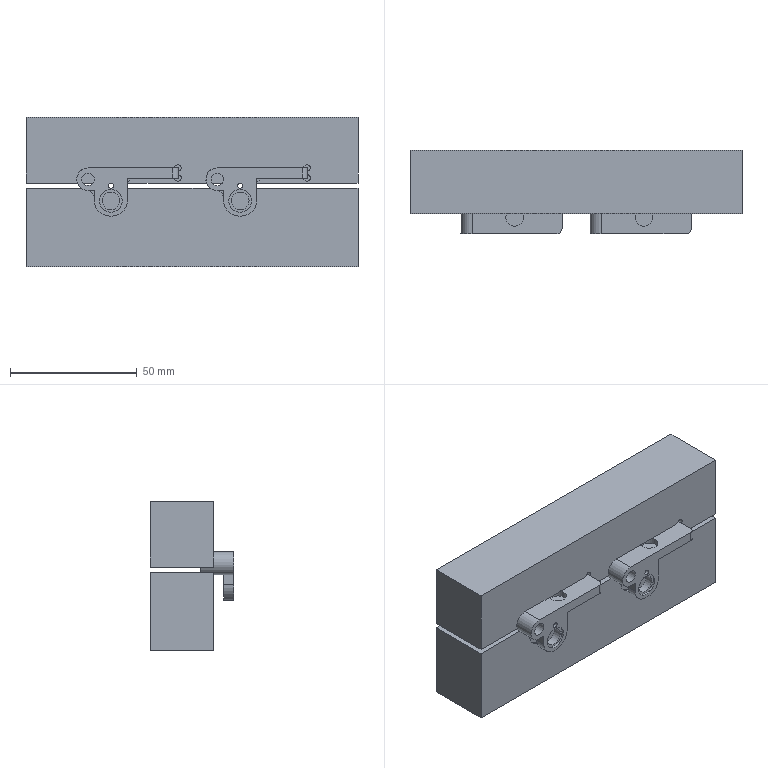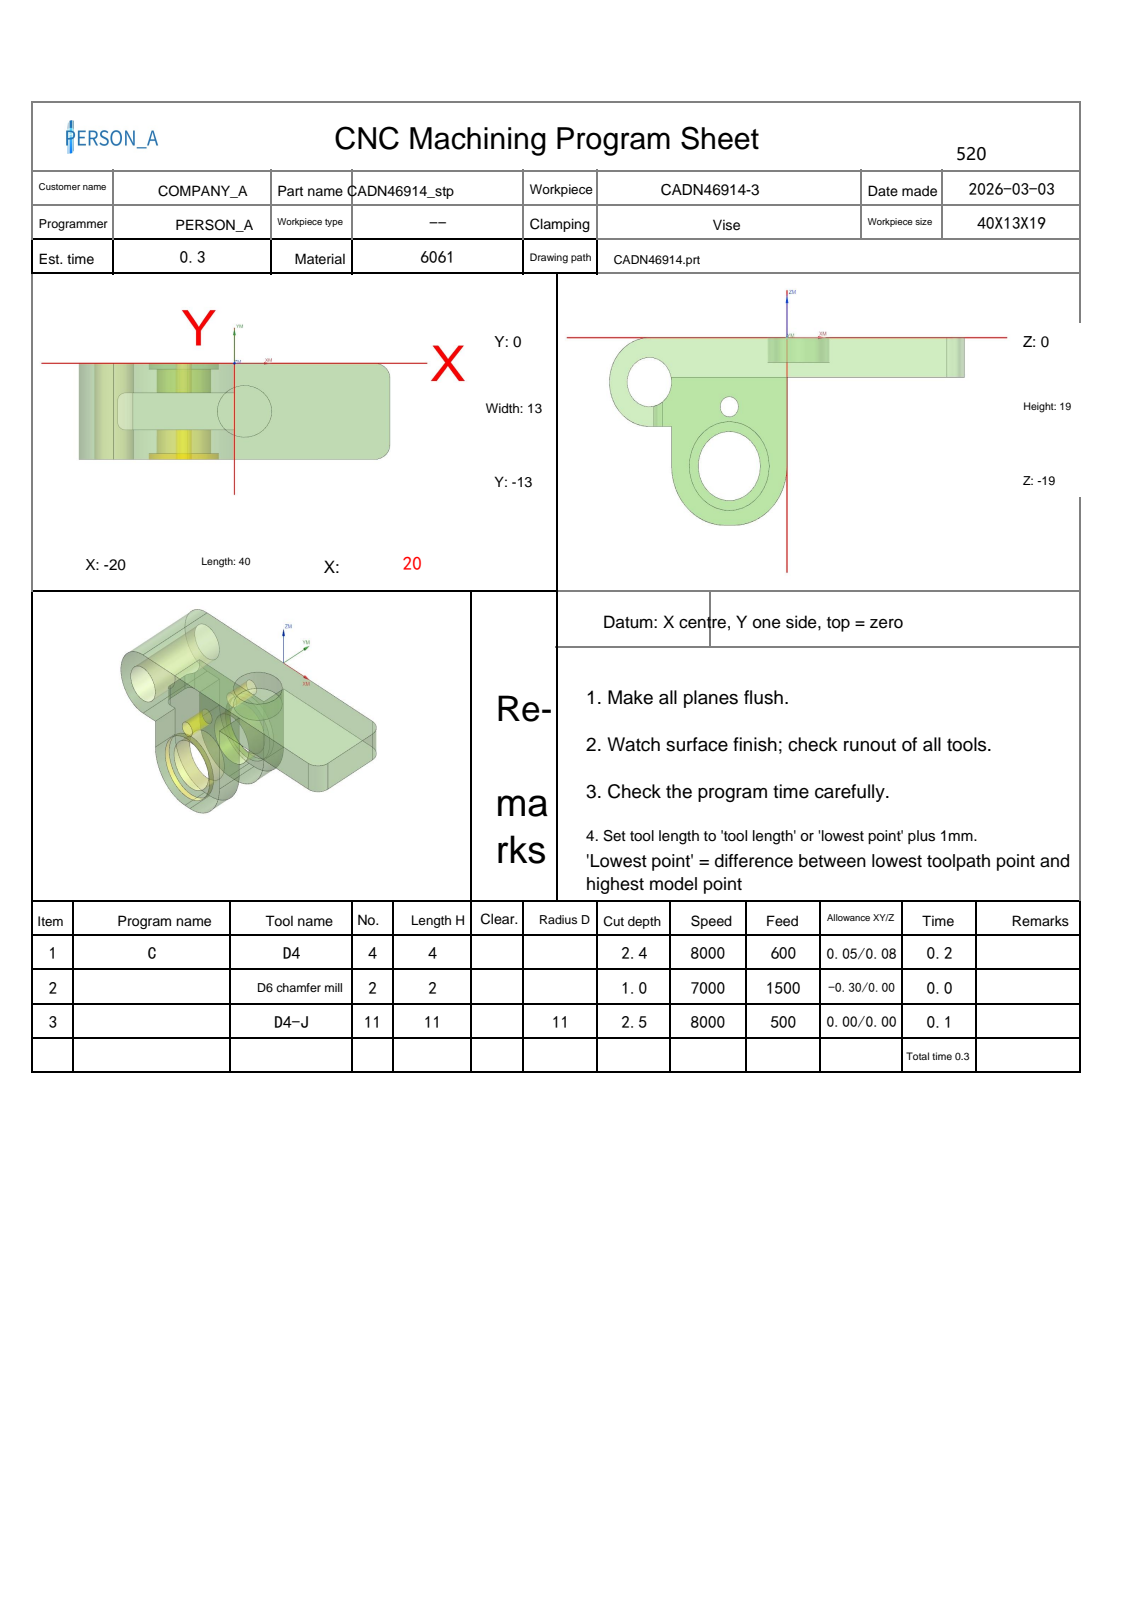NC program | NX | posted by the shop | part box 131 x 33 x 59 mm
Whole program:
%
O0001
(Machine time: 0.90 MIN)
(===Total Tool:3===)
(T4=D4      D=4.   R=0.   D-  H04 Z=-2.44 )
(T2=D6 chamfer mill   D=6.   R=0.   D-  H02 Z=-1.   )
(T11=D4-J   D=4.   R=0.   D11 H11 Z=-2.5  )
G80 G90 G17 G49 G40
G91 G28 Z0
M01
N1 T04 M06
(D4  D=4. R=0. H=04 ce=0.05 di=0.08)
G00 G90 G54 X2.509 Y-5.655 M03 S8000
G43 H04 Z50.
M08
Z.8
G01 X2.124 Y-5.271 Z.771 F600.
X1.596 Y-5.05 Z.742
X1.004 Z.71
X.476 Y-5.271 Z.68
X.071 Y-5.676 Z.65
X-.15 Y-6.204 Z.62
Y-6.796 Z.589
X.207 Y-7.498 Z.548
X.687 Y-7.847 Z.517
X1.004 Y-7.95 Z.5
X1.596 Z.468
X2.124 Y-7.729 Z.439
X2.529 Y-7.324 Z.409
X2.75 Y-6.796 Z.379
Y-6.204 Z.347
X2.529 Y-5.676 Z.317
X2.124 Y-5.271 Z.287
X1.596 Y-5.05 Z.257
X1.004 Z.226
X.476 Y-5.271 Z.196
X.071 Y-5.676 Z.166
X-.15 Y-6.204 Z.136
Y-6.796 Z.105
X.207 Y-7.498 Z.064
X.687 Y-7.847 Z.033
X1.004 Y-7.95 Z.016
X1.3 Z0.0
G03 X2.75 Y-6.5 Z-.068 I0.0 J1.45
X1.3 Y-5.05 Z-.136 I-1.45 J0.0
X-.15 Y-6.5 Z-.203 I0.0 J-1.45
X.447 Y-7.673 Z-.244 I1.45 J0.0
X1.3 Y-7.95 Z-.271 I.853 J1.173
X2.75 Y-6.5 Z-.339 I0.0 J1.45
X1.3 Y-5.05 Z-.407 I-1.45 J0.0
X-.15 Y-6.5 Z-.474 I0.0 J-1.45
X.447 Y-7.673 Z-.515 I1.45 J0.0
X1.3 Y-7.95 Z-.542 I.853 J1.173
X2.75 Y-6.5 Z-.61 I0.0 J1.45
X1.3 Y-5.05 Z-.678 I-1.45 J0.0
X-.15 Y-6.5 Z-.746 I0.0 J-1.45
X.447 Y-7.673 Z-.786 I1.45 J0.0
X1.3 Y-7.95 Z-.813 I.853 J1.173
X2.75 Y-6.5 Z-.881 I0.0 J1.45
X1.3 Y-5.05 Z-.949 I-1.45 J0.0
X-.15 Y-6.5 Z-1.017 I0.0 J-1.45
X.447 Y-7.673 Z-1.057 I1.45 J0.0
X1.3 Y-7.95 Z-1.084 I.853 J1.173
X2.75 Y-6.5 Z-1.152 I0.0 J1.45
X1.3 Y-5.05 Z-1.22 I-1.45 J0.0
X-.15 Y-6.5 Z-1.288 I0.0 J-1.45
X.447 Y-7.673 Z-1.328 I1.45 J0.0
X1.3 Y-7.95 Z-1.356 I.853 J1.173
X2.75 Y-6.5 Z-1.423 I0.0 J1.45
X1.3 Y-5.05 Z-1.491 I-1.45 J0.0
X-.15 Y-6.5 Z-1.559 I0.0 J-1.45
X.447 Y-7.673 Z-1.6 I1.45 J0.0
X1.3 Y-7.95 Z-1.627 I.853 J1.173
X2.75 Y-6.5 Z-1.694 I0.0 J1.45
X1.3 Y-5.05 Z-1.762 I-1.45 J0.0
X-.15 Y-6.5 Z-1.83 I0.0 J-1.45
X.447 Y-7.673 Z-1.871 I1.45 J0.0
X1.3 Y-7.95 Z-1.898 I.853 J1.173
X2.75 Y-6.5 Z-1.966 I0.0 J1.45
X1.3 Y-5.05 Z-2.033 I-1.45 J0.0
X-.15 Y-6.5 Z-2.101 I0.0 J-1.45
X.447 Y-7.673 Z-2.142 I1.45 J0.0
X1.3 Y-7.95 Z-2.169 I.853 J1.173
X2.75 Y-6.5 Z-2.237 I0.0 J1.45
X1.3 Y-5.05 Z-2.304 I-1.45 J0.0
X-.15 Y-6.5 Z-2.372 I0.0 J-1.45
X.447 Y-7.673 Z-2.413 I1.45 J0.0
X1.3 Y-7.95 Z-2.44 I.853 J1.173
X2.75 Y-6.5 I0.0 J1.45
X1.3 Y-5.05 I-1.45 J0.0
X-.15 Y-6.5 I0.0 J-1.45
X1.3 Y-7.95 I1.45 J0.0
X1.695 Y-7.895 I0.0 J1.45
G01 Z-1.64
G00 Z50.
G91 G28 Z0.0
M05
M09
G91 G28 Z0.0
M01
N2 T02 M06
(D6 chamfer mill  D=6. R=0. H=02 ce=-0.30 di=0.00)
G00 G90 G54 X-1.38 Y-5.697 M03 S7000
G43 H02 Z50.
M08
Z2.5
G01 X-1.416 Y-5.806 Z2.458 F1500.
X-1.481 Y-6.15 Z2.331
X-1.503 Y-6.5 Z2.203
X-1.481 Y-6.85 Z2.075
X-1.416 Y-7.194 Z1.948
X-1.308 Y-7.528 Z1.82
X-1.159 Y-7.845 Z1.693
X-.972 Y-8.141 Z1.565
X-.75 Y-8.412 Z1.438
X-.495 Y-8.653 Z1.31
X-.212 Y-8.86 Z1.183
X.012 Y-8.99 Z1.088
X.333 Y-9.131 Z.961
X.669 Y-9.231 Z.833
X1.015 Y-9.288 Z.705
X1.365 Y-9.302 Z.578
X1.714 Y-9.272 Z.45
X2.057 Y-9.199 Z.323
X2.388 Y-9.083 Z.195
X2.702 Y-8.927 Z.068
X2.993 Y-8.734 Z-.06
X3.259 Y-8.505 Z-.187
X3.494 Y-8.245 Z-.315
X3.694 Y-7.957 Z-.443
X3.858 Y-7.647 Z-.57
X3.981 Y-7.319 Z-.698
X4.062 Y-6.978 Z-.825
X4.1 Y-6.63 Z-.953
Y-6.5 Z-1.
G03 X1.3 Y-3.7 I-2.8 J0.0
X-1.5 Y-6.5 I0.0 J-2.8
X1.3 Y-9.3 I2.8 J0.0
X4.1 Y-6.5 I0.0 J2.8
X4.055 Y-6.003 I-2.8 J0.0
G01 Z1.5
G00 Z50.
G91 G28 Z0.0
M05
M09
G91 G28 Z0.0
M01
N3 T11 M06
(D4-J  D=4. R=0. H=11 ce=0.00 di=0.00)
G00 G90 G54 X1.65 Y-5.082 M03 S8000
G43 H11 Z50.
M08
Z.5
G01 X1.456 Y-5.038 Z.49 F500.
X1.179 Y-5.035 Z.475
X.889 Y-5.089 Z.46
X.616 Y-5.199 Z.444
X.37 Y-5.362 Z.429
X.162 Y-5.57 Z.413
X-.001 Y-5.816 Z.398
X-.111 Y-6.089 Z.382
X-.165 Y-6.379 Z.367
Y-6.621 Z.354
X-.111 Y-6.911 Z.339
X-.001 Y-7.184 Z.323
X.162 Y-7.43 Z.308
X.37 Y-7.638 Z.292
X.616 Y-7.801 Z.277
X.889 Y-7.911 Z.262
X1.179 Y-7.965 Z.246
X1.421 Z.233
X1.711 Y-7.911 Z.218
X1.984 Y-7.801 Z.202
X2.23 Y-7.638 Z.187
X2.438 Y-7.43 Z.172
X2.601 Y-7.184 Z.156
X2.711 Y-6.911 Z.141
X2.765 Y-6.621 Z.125
Y-6.379 Z.113
X2.699 Y-6.048 Z.095
X2.559 Y-5.74 Z.077
X2.352 Y-5.473 Z.059
X2.09 Y-5.26 Z.042
X1.786 Y-5.113 Z.024
X1.456 Y-5.038 Z.006
X1.335 Y-5.035 Z0.0
G41 D11
X1.3 Y-5.
G03 X-.2 Y-6.5 Z-.313 I0.0 J-1.5
X1.3 Y-8. Z-.625 I1.5 J0.0
X2.8 Y-6.5 Z-.938 I0.0 J1.5
X1.3 Y-5. Z-1.25 I-1.5 J0.0
X-.2 Y-6.5 Z-1.563 I0.0 J-1.5
X1.3 Y-8. Z-1.875 I1.5 J0.0
X2.8 Y-6.5 Z-2.188 I0.0 J1.5
X1.3 Y-5. Z-2.5 I-1.5 J0.0
X-.2 Y-6.5 I0.0 J-1.5
X1.3 Y-8. I1.5 J0.0
X2.8 Y-6.5 I0.0 J1.5
X1.3 Y-5. I-1.5 J0.0
X.905 Y-5.053 I0.0 J-1.5
G01 X.879 Y-5.063
X.865 Y-5.087
X.87 Y-5.114
G40 X.883 Y-5.163
Z-1.5
G00 Z50.
M05
M09
G91 G28 Z0.0
G91 G28 Y0.0
M30
%